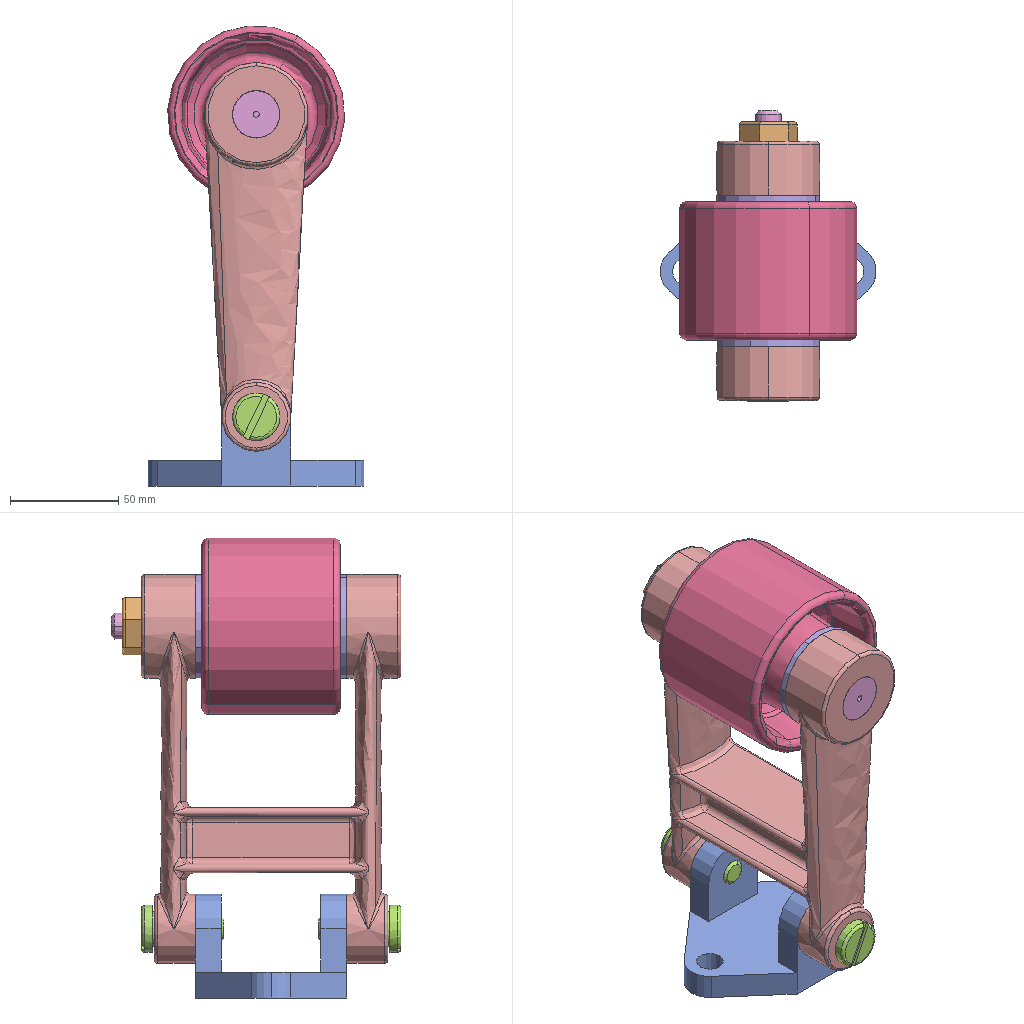Assembly | SolidWorks | 9 different items | 11 placed | box 100 x 134 x 213 mm
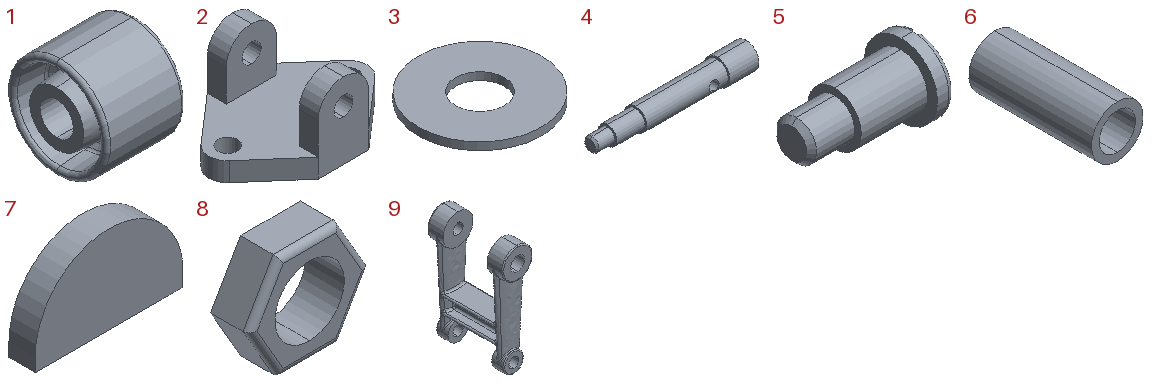Parts list (item | quantity | size | volume | features):
1 | x1 | 64 x 82 x 82 mm | 200004 mm3 | features Revolution 1
2 | x1 | 99.999 x 70 x 48 mm | 79061 mm3 | features Cut 2, Boss 1, Extrusion 1, Fillet 1
3 | x2 | 48 x 48 x 3 mm | 4578 mm3 | features Extrusion 1
4 | x1 | 134 x 22 x 22 mm | 34206 mm3 | features Cut 2, Chamfer 1, RevCut 1, Revolution 1
5 | x2 | 38 x 22 x 22 mm | 7225 mm3 | features Chamfer 1, Cut 1, Fillet 1, Revolution 1
6 | x1 | 27 x 64 x 27 mm | 18498 mm3 | features Extrusion 1
7 | x1 | 18 x 3.2 x 10.7 mm | 505.07 mm3 | features Extrusion 1
8 | x1 | 27.713 x 9 x 24 mm | 2641 mm3 | features Extrusion 1, Fillet 1
9 | x1 | 48 x 120 x 180 mm | 208513 mm3 | features Boss 7, Cut 3, Fillet 3, Blend 2
Mates (type | each side: item.copy, entity, surface, feature):
Parallel | 9.1 face plane Extrude5 | 2.1 face plane Extrude1
Parallel | 9.1 axis | 2.1 axis
Coincident | 9.1 face plane Extrude4 | 2.1 face plane Extrude1
Coincident | 9.1 axis | 2.1 axis
Parallel | 9.1 axis | 5.1 axis
Coincident | 2.1 face plane Extrude1 | 5.1 face plane Revolve1
Coincident | 9.1 axis | 5.1 axis
Parallel | 9.1 axis | 5.2 axis
Coincident | 2.1 face plane Extrude1 | 5.2 face plane Revolve1
Coincident | 9.1 axis | 5.2 axis
Parallel | 4.1 face plane Cut-Revolve3 | 7.1 face plane Extrude1
Concentric | 4.1 face cylinder Cut-Revolve3 | 7.1 face cylinder Extrude1
Parallel | 4.1 edge | 7.1 face plane Extrude1
Coincident | 4.1 face plane Cut-Revolve3 | 7.1 face plane Extrude1
Parallel | 9.1 axis | 4.1 axis
Coincident | 9.1 face plane Extrude1 | 4.1 face plane Revolve1
Parallel | 9.1 edge | 7.1 edge
Parallel | 9.1 face plane Cut-Extrude3 | 7.1 face plane Extrude1
Concentric | 9.1 edge | 4.1 edge
Parallel | 4.1 axis | 8.1 axis
Coincident | 4.1 axis | 8.1 axis
Coincident | 9.1 face plane Extrude2 | 8.1 face plane Extrude1
Parallel | 9.1 face plane Extrude1 | 3.1 face plane Extrude1
Coincident | 9.1 axis | 3.1 axis
Coincident | 9.1 face plane Extrude1 | 3.1 face plane Extrude1
Parallel | 4.1 axis | 3.2 axis
Coincident | 9.1 face plane Extrude4 | 3.2 face plane Extrude1
Coincident | 4.1 axis | 3.2 axis
Parallel | 4.1 axis | 6.1 axis
Coincident | 3.2 face plane Extrude1 | 6.1 face plane Extrude1
Coincident | 4.1 axis | 6.1 axis
Parallel | 3.1 face plane Extrude1 | 1.1 face plane Revolve1
Coincident | 4.1 axis | 1.1 axis
Coincident | 3.2 face plane Extrude1 | 1.1 face plane Revolve1